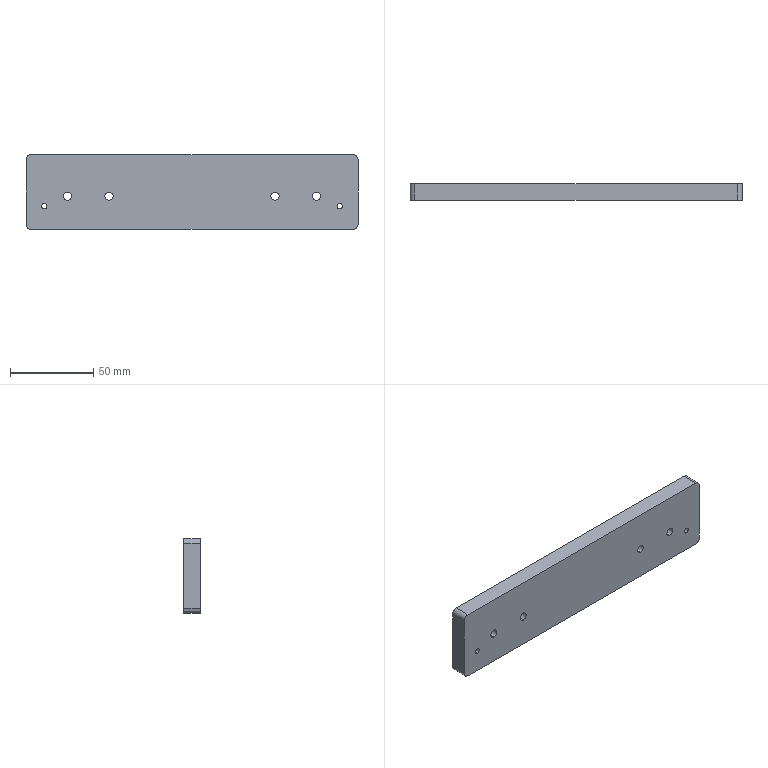Part | SolidWorks | features HoleWzd 2, MoveFace 2, Extrusion 1, Fillet 1 | 1 solid | 22 faces | box 200 x 10 x 45 mm | volume 88966 mm3 | cylinder 16 | plane 6 | commonest cylinder face diameters 5 x8 3.3 x4 6 x4
STEP:
#1=CARTESIAN_POINT('',(-75.,0.,-2.5));
#2=VERTEX_POINT('',#1);
#3=CARTESIAN_POINT('',(-75.,0.,2.5));
#4=VERTEX_POINT('',#3);
#5=CARTESIAN_POINT('',(-75.,0.,0.));
#6=DIRECTION('',(0.,1.,0.));
#7=DIRECTION('',(0.,0.,1.));
#8=AXIS2_PLACEMENT_3D('',#5,#6,#7);
#9=CIRCLE('',#8,2.5);
#10=EDGE_CURVE('',#2,#4,#9,.T.);
#11=ORIENTED_EDGE('',*,*,#10,.F.);
#12=CARTESIAN_POINT('',(-75.,10.,-2.5));
#13=VERTEX_POINT('',#12);
#14=CARTESIAN_POINT('',(-75.,10.,-2.5));
#15=DIRECTION('',(0.,1.,0.));
#16=VECTOR('',#15,1000.);
#17=LINE('',#14,#16);
#18=EDGE_CURVE('',#2,#13,#17,.T.);
#19=ORIENTED_EDGE('',*,*,#18,.T.);
#20=CARTESIAN_POINT('',(-75.,10.,2.5));
#21=VERTEX_POINT('',#20);
#22=CARTESIAN_POINT('',(-75.,10.,0.));
#23=DIRECTION('',(0.,1.,0.));
#24=DIRECTION('',(0.,0.,1.));
#25=AXIS2_PLACEMENT_3D('',#22,#23,#24);
#26=CIRCLE('',#25,2.5);
#27=EDGE_CURVE('',#13,#21,#26,.T.);
#28=ORIENTED_EDGE('',*,*,#27,.T.);
#29=CARTESIAN_POINT('',(-75.,10.,2.5));
#30=DIRECTION('',(0.,1.,0.));
#31=VECTOR('',#30,1000.);
#32=LINE('',#29,#31);
#33=EDGE_CURVE('',#4,#21,#32,.T.);
#34=ORIENTED_EDGE('',*,*,#33,.F.);
#35=EDGE_LOOP('',(#11,#19,#28,#34));
#36=FACE_OUTER_BOUND('',#35,.T.);
#37=CARTESIAN_POINT('',(-75.,10.,0.));
#38=DIRECTION('',(0.,1.,0.));
#39=DIRECTION('',(0.,0.,1.));
#40=AXIS2_PLACEMENT_3D('',#37,#38,#39);
#41=CYLINDRICAL_SURFACE('',#40,2.5);
#42=ADVANCED_FACE('',(#36),#41,.F.);
#43=CARTESIAN_POINT('',(75.,0.,-2.5));
#44=VERTEX_POINT('',#43);
#45=CARTESIAN_POINT('',(75.,0.,2.5));
#46=VERTEX_POINT('',#45);
#47=CARTESIAN_POINT('',(75.,0.,0.));
#48=DIRECTION('',(0.,1.,0.));
#49=DIRECTION('',(0.,0.,1.));
#50=AXIS2_PLACEMENT_3D('',#47,#48,#49);
#51=CIRCLE('',#50,2.5);
#52=EDGE_CURVE('',#44,#46,#51,.T.);
#53=ORIENTED_EDGE('',*,*,#52,.F.);
#54=CARTESIAN_POINT('',(75.,10.,-2.5));
#55=VERTEX_POINT('',#54);
#56=CARTESIAN_POINT('',(75.,10.,-2.5));
#57=DIRECTION('',(0.,1.,0.));
#58=VECTOR('',#57,1000.);
#59=LINE('',#56,#58);
#60=EDGE_CURVE('',#44,#55,#59,.T.);
#61=ORIENTED_EDGE('',*,*,#60,.T.);
#62=CARTESIAN_POINT('',(75.,10.,2.5));
#63=VERTEX_POINT('',#62);
#64=CARTESIAN_POINT('',(75.,10.,0.));
#65=DIRECTION('',(0.,1.,0.));
#66=DIRECTION('',(0.,0.,1.));
#67=AXIS2_PLACEMENT_3D('',#64,#65,#66);
#68=CIRCLE('',#67,2.5);
#69=EDGE_CURVE('',#55,#63,#68,.T.);
#70=ORIENTED_EDGE('',*,*,#69,.T.);
#71=CARTESIAN_POINT('',(75.,10.,2.5));
#72=DIRECTION('',(0.,1.,0.));
#73=VECTOR('',#72,1000.);
#74=LINE('',#71,#73);
#75=EDGE_CURVE('',#46,#63,#74,.T.);
#76=ORIENTED_EDGE('',*,*,#75,.F.);
#77=EDGE_LOOP('',(#53,#61,#70,#76));
#78=FACE_OUTER_BOUND('',#77,.T.);
#79=CARTESIAN_POINT('',(75.,10.,0.));
#80=DIRECTION('',(0.,1.,0.));
#81=DIRECTION('',(0.,0.,1.));
#82=AXIS2_PLACEMENT_3D('',#79,#80,#81);
#83=CYLINDRICAL_SURFACE('',#82,2.5);
#84=ADVANCED_FACE('',(#78),#83,.F.);
#85=CARTESIAN_POINT('',(-50.,0.,-2.5));
#86=VERTEX_POINT('',#85);
#87=CARTESIAN_POINT('',(-50.,0.,2.5));
#88=VERTEX_POINT('',#87);
#89=CARTESIAN_POINT('',(-50.,0.,0.));
#90=DIRECTION('',(0.,1.,0.));
#91=DIRECTION('',(0.,0.,1.));
#92=AXIS2_PLACEMENT_3D('',#89,#90,#91);
#93=CIRCLE('',#92,2.5);
#94=EDGE_CURVE('',#86,#88,#93,.T.);
#95=ORIENTED_EDGE('',*,*,#94,.F.);
#96=CARTESIAN_POINT('',(-50.,10.,-2.5));
#97=VERTEX_POINT('',#96);
#98=CARTESIAN_POINT('',(-50.,10.,-2.5));
#99=DIRECTION('',(0.,1.,0.));
#100=VECTOR('',#99,1000.);
#101=LINE('',#98,#100);
#102=EDGE_CURVE('',#86,#97,#101,.T.);
#103=ORIENTED_EDGE('',*,*,#102,.T.);
#104=CARTESIAN_POINT('',(-50.,10.,2.5));
#105=VERTEX_POINT('',#104);
#106=CARTESIAN_POINT('',(-50.,10.,0.));
#107=DIRECTION('',(0.,1.,0.));
#108=DIRECTION('',(0.,0.,1.));
#109=AXIS2_PLACEMENT_3D('',#106,#107,#108);
#110=CIRCLE('',#109,2.5);
#111=EDGE_CURVE('',#97,#105,#110,.T.);
#112=ORIENTED_EDGE('',*,*,#111,.T.);
#113=CARTESIAN_POINT('',(-50.,10.,2.5));
#114=DIRECTION('',(0.,1.,0.));
#115=VECTOR('',#114,1000.);
#116=LINE('',#113,#115);
#117=EDGE_CURVE('',#88,#105,#116,.T.);
#118=ORIENTED_EDGE('',*,*,#117,.F.);
#119=EDGE_LOOP('',(#95,#103,#112,#118));
#120=FACE_OUTER_BOUND('',#119,.T.);
#121=CARTESIAN_POINT('',(-50.,10.,0.));
#122=DIRECTION('',(0.,1.,0.));
#123=DIRECTION('',(0.,0.,1.));
#124=AXIS2_PLACEMENT_3D('',#121,#122,#123);
#125=CYLINDRICAL_SURFACE('',#124,2.5);
#126=ADVANCED_FACE('',(#120),#125,.F.);
#127=CARTESIAN_POINT('',(50.,0.,-2.5));
#128=VERTEX_POINT('',#127);
#129=CARTESIAN_POINT('',(50.,0.,2.5));
#130=VERTEX_POINT('',#129);
#131=CARTESIAN_POINT('',(50.,0.,0.));
#132=DIRECTION('',(0.,1.,0.));
#133=DIRECTION('',(0.,0.,1.));
#134=AXIS2_PLACEMENT_3D('',#131,#132,#133);
#135=CIRCLE('',#134,2.5);
#136=EDGE_CURVE('',#128,#130,#135,.T.);
#137=ORIENTED_EDGE('',*,*,#136,.F.);
#138=CARTESIAN_POINT('',(50.,10.,-2.5));
#139=VERTEX_POINT('',#138);
#140=CARTESIAN_POINT('',(50.,10.,-2.5));
#141=DIRECTION('',(0.,1.,0.));
#142=VECTOR('',#141,1000.);
#143=LINE('',#140,#142);
#144=EDGE_CURVE('',#128,#139,#143,.T.);
#145=ORIENTED_EDGE('',*,*,#144,.T.);
#146=CARTESIAN_POINT('',(50.,10.,2.5));
#147=VERTEX_POINT('',#146);
#148=CARTESIAN_POINT('',(50.,10.,0.));
#149=DIRECTION('',(0.,1.,0.));
#150=DIRECTION('',(0.,0.,1.));
#151=AXIS2_PLACEMENT_3D('',#148,#149,#150);
#152=CIRCLE('',#151,2.5);
#153=EDGE_CURVE('',#139,#147,#152,.T.);
#154=ORIENTED_EDGE('',*,*,#153,.T.);
#155=CARTESIAN_POINT('',(50.,10.,2.5));
#156=DIRECTION('',(0.,1.,0.));
#157=VECTOR('',#156,1000.);
#158=LINE('',#155,#157);
#159=EDGE_CURVE('',#130,#147,#158,.T.);
#160=ORIENTED_EDGE('',*,*,#159,.F.);
#161=EDGE_LOOP('',(#137,#145,#154,#160));
#162=FACE_OUTER_BOUND('',#161,.T.);
#163=CARTESIAN_POINT('',(50.,10.,0.));
#164=DIRECTION('',(0.,1.,0.));
#165=DIRECTION('',(0.,0.,1.));
#166=AXIS2_PLACEMENT_3D('',#163,#164,#165);
#167=CYLINDRICAL_SURFACE('',#166,2.5);
#168=ADVANCED_FACE('',(#162),#167,.F.);
#169=CARTESIAN_POINT('',(-89.,0.,-7.65));
#170=VERTEX_POINT('',#169);
#171=CARTESIAN_POINT('',(-89.,0.,-4.35));
#172=VERTEX_POINT('',#171);
#173=CARTESIAN_POINT('',(-89.,0.,-6.));
#174=DIRECTION('',(0.,1.,0.));
#175=DIRECTION('',(0.,0.,1.));
#176=AXIS2_PLACEMENT_3D('',#173,#174,#175);
#177=CIRCLE('',#176,1.65);
#178=EDGE_CURVE('',#170,#172,#177,.T.);
#179=ORIENTED_EDGE('',*,*,#178,.F.);
#180=CARTESIAN_POINT('',(-89.,10.,-7.65));
#181=VERTEX_POINT('',#180);
#182=CARTESIAN_POINT('',(-89.,10.,-7.65));
#183=DIRECTION('',(0.,1.,0.));
#184=VECTOR('',#183,1000.);
#185=LINE('',#182,#184);
#186=EDGE_CURVE('',#170,#181,#185,.T.);
#187=ORIENTED_EDGE('',*,*,#186,.T.);
#188=CARTESIAN_POINT('',(-89.,10.,-4.35));
#189=VERTEX_POINT('',#188);
#190=CARTESIAN_POINT('',(-89.,10.,-6.));
#191=DIRECTION('',(0.,1.,0.));
#192=DIRECTION('',(0.,0.,1.));
#193=AXIS2_PLACEMENT_3D('',#190,#191,#192);
#194=CIRCLE('',#193,1.65);
#195=EDGE_CURVE('',#181,#189,#194,.T.);
#196=ORIENTED_EDGE('',*,*,#195,.T.);
#197=CARTESIAN_POINT('',(-89.,10.,-4.35));
#198=DIRECTION('',(0.,1.,0.));
#199=VECTOR('',#198,1000.);
#200=LINE('',#197,#199);
#201=EDGE_CURVE('',#172,#189,#200,.T.);
#202=ORIENTED_EDGE('',*,*,#201,.F.);
#203=EDGE_LOOP('',(#179,#187,#196,#202));
#204=FACE_OUTER_BOUND('',#203,.T.);
#205=CARTESIAN_POINT('',(-89.,10.,-6.));
#206=DIRECTION('',(0.,1.,0.));
#207=DIRECTION('',(0.,0.,1.));
#208=AXIS2_PLACEMENT_3D('',#205,#206,#207);
#209=CYLINDRICAL_SURFACE('',#208,1.65);
#210=ADVANCED_FACE('',(#204),#209,.F.);
#211=CARTESIAN_POINT('',(89.,0.,-7.65));
#212=VERTEX_POINT('',#211);
#213=CARTESIAN_POINT('',(89.,0.,-4.35));
#214=VERTEX_POINT('',#213);
#215=CARTESIAN_POINT('',(89.,0.,-6.));
#216=DIRECTION('',(0.,1.,0.));
#217=DIRECTION('',(0.,0.,1.));
#218=AXIS2_PLACEMENT_3D('',#215,#216,#217);
#219=CIRCLE('',#218,1.65);
#220=EDGE_CURVE('',#212,#214,#219,.T.);
#221=ORIENTED_EDGE('',*,*,#220,.F.);
#222=CARTESIAN_POINT('',(89.,10.,-7.65));
#223=VERTEX_POINT('',#222);
#224=CARTESIAN_POINT('',(89.,10.,-7.65));
#225=DIRECTION('',(0.,1.,0.));
#226=VECTOR('',#225,1000.);
#227=LINE('',#224,#226);
#228=EDGE_CURVE('',#212,#223,#227,.T.);
#229=ORIENTED_EDGE('',*,*,#228,.T.);
#230=CARTESIAN_POINT('',(89.,10.,-4.35));
#231=VERTEX_POINT('',#230);
#232=CARTESIAN_POINT('',(89.,10.,-6.));
#233=DIRECTION('',(0.,1.,0.));
#234=DIRECTION('',(0.,0.,1.));
#235=AXIS2_PLACEMENT_3D('',#232,#233,#234);
#236=CIRCLE('',#235,1.65);
#237=EDGE_CURVE('',#223,#231,#236,.T.);
#238=ORIENTED_EDGE('',*,*,#237,.T.);
#239=CARTESIAN_POINT('',(89.,10.,-4.35));
#240=DIRECTION('',(0.,1.,0.));
#241=VECTOR('',#240,1000.);
#242=LINE('',#239,#241);
#243=EDGE_CURVE('',#214,#231,#242,.T.);
#244=ORIENTED_EDGE('',*,*,#243,.F.);
#245=EDGE_LOOP('',(#221,#229,#238,#244));
#246=FACE_OUTER_BOUND('',#245,.T.);
#247=CARTESIAN_POINT('',(89.,10.,-6.));
#248=DIRECTION('',(0.,1.,0.));
#249=DIRECTION('',(0.,0.,1.));
#250=AXIS2_PLACEMENT_3D('',#247,#248,#249);
#251=CYLINDRICAL_SURFACE('',#250,1.65);
#252=ADVANCED_FACE('',(#246),#251,.F.);
#253=CARTESIAN_POINT('',(-75.,10.,0.));
#254=DIRECTION('',(0.,1.,0.));
#255=DIRECTION('',(0.,0.,1.));
#256=AXIS2_PLACEMENT_3D('',#253,#254,#255);
#257=CIRCLE('',#256,2.5);
#258=EDGE_CURVE('',#21,#13,#257,.T.);
#259=ORIENTED_EDGE('',*,*,#258,.F.);
#260=ORIENTED_EDGE('',*,*,#27,.F.);
#261=EDGE_LOOP('',(#259,#260));
#262=FACE_BOUND('',#261,.T.);
#263=CARTESIAN_POINT('',(75.,10.,0.));
#264=DIRECTION('',(0.,1.,0.));
#265=DIRECTION('',(0.,0.,1.));
#266=AXIS2_PLACEMENT_3D('',#263,#264,#265);
#267=CIRCLE('',#266,2.5);
#268=EDGE_CURVE('',#63,#55,#267,.T.);
#269=ORIENTED_EDGE('',*,*,#268,.F.);
#270=ORIENTED_EDGE('',*,*,#69,.F.);
#271=EDGE_LOOP('',(#269,#270));
#272=FACE_BOUND('',#271,.T.);
#273=CARTESIAN_POINT('',(-50.,10.,0.));
#274=DIRECTION('',(0.,1.,0.));
#275=DIRECTION('',(0.,0.,1.));
#276=AXIS2_PLACEMENT_3D('',#273,#274,#275);
#277=CIRCLE('',#276,2.5);
#278=EDGE_CURVE('',#105,#97,#277,.T.);
#279=ORIENTED_EDGE('',*,*,#278,.F.);
#280=ORIENTED_EDGE('',*,*,#111,.F.);
#281=EDGE_LOOP('',(#279,#280));
#282=FACE_BOUND('',#281,.T.);
#283=CARTESIAN_POINT('',(50.,10.,0.));
#284=DIRECTION('',(0.,1.,0.));
#285=DIRECTION('',(0.,0.,1.));
#286=AXIS2_PLACEMENT_3D('',#283,#284,#285);
#287=CIRCLE('',#286,2.5);
#288=EDGE_CURVE('',#147,#139,#287,.T.);
#289=ORIENTED_EDGE('',*,*,#288,.F.);
#290=ORIENTED_EDGE('',*,*,#153,.F.);
#291=EDGE_LOOP('',(#289,#290));
#292=FACE_BOUND('',#291,.T.);
#293=CARTESIAN_POINT('',(89.,10.,-6.));
#294=DIRECTION('',(0.,1.,0.));
#295=DIRECTION('',(0.,0.,1.));
#296=AXIS2_PLACEMENT_3D('',#293,#294,#295);
#297=CIRCLE('',#296,1.65);
#298=EDGE_CURVE('',#231,#223,#297,.T.);
#299=ORIENTED_EDGE('',*,*,#298,.F.);
#300=ORIENTED_EDGE('',*,*,#237,.F.);
#301=EDGE_LOOP('',(#299,#300));
#302=FACE_BOUND('',#301,.T.);
#303=CARTESIAN_POINT('',(100.,10.,22.));
#304=VERTEX_POINT('',#303);
#305=CARTESIAN_POINT('',(100.,10.,-17.));
#306=VERTEX_POINT('',#305);
#307=CARTESIAN_POINT('',(100.,10.,10.));
#308=DIRECTION('',(0.,0.,-1.));
#309=VECTOR('',#308,1000.);
#310=LINE('',#307,#309);
#311=EDGE_CURVE('',#304,#306,#310,.T.);
#312=ORIENTED_EDGE('',*,*,#311,.T.);
#313=CARTESIAN_POINT('',(97.,10.,-20.));
#314=VERTEX_POINT('',#313);
#315=CARTESIAN_POINT('',(97.,10.,-17.));
#316=DIRECTION('',(0.,1.,0.));
#317=DIRECTION('',(0.,0.,-1.));
#318=AXIS2_PLACEMENT_3D('',#315,#316,#317);
#319=CIRCLE('',#318,3.);
#320=EDGE_CURVE('',#306,#314,#319,.T.);
#321=ORIENTED_EDGE('',*,*,#320,.T.);
#322=CARTESIAN_POINT('',(-97.,10.,-20.));
#323=VERTEX_POINT('',#322);
#324=CARTESIAN_POINT('',(-100.,10.,-20.));
#325=DIRECTION('',(-1.,0.,0.));
#326=VECTOR('',#325,1000.);
#327=LINE('',#324,#326);
#328=EDGE_CURVE('',#314,#323,#327,.T.);
#329=ORIENTED_EDGE('',*,*,#328,.T.);
#330=CARTESIAN_POINT('',(-100.,10.,-17.));
#331=VERTEX_POINT('',#330);
#332=CARTESIAN_POINT('',(-97.,10.,-17.));
#333=DIRECTION('',(0.,1.,0.));
#334=DIRECTION('',(0.,0.,-1.));
#335=AXIS2_PLACEMENT_3D('',#332,#333,#334);
#336=CIRCLE('',#335,3.);
#337=EDGE_CURVE('',#323,#331,#336,.T.);
#338=ORIENTED_EDGE('',*,*,#337,.T.);
#339=CARTESIAN_POINT('',(-100.,10.,22.));
#340=VERTEX_POINT('',#339);
#341=CARTESIAN_POINT('',(-100.,10.,10.));
#342=DIRECTION('',(0.,0.,1.));
#343=VECTOR('',#342,1000.);
#344=LINE('',#341,#343);
#345=EDGE_CURVE('',#331,#340,#344,.T.);
#346=ORIENTED_EDGE('',*,*,#345,.T.);
#347=CARTESIAN_POINT('',(-97.,10.,25.));
#348=VERTEX_POINT('',#347);
#349=CARTESIAN_POINT('',(-97.,10.,22.));
#350=DIRECTION('',(0.,1.,0.));
#351=DIRECTION('',(0.,0.,-1.));
#352=AXIS2_PLACEMENT_3D('',#349,#350,#351);
#353=CIRCLE('',#352,3.);
#354=EDGE_CURVE('',#340,#348,#353,.T.);
#355=ORIENTED_EDGE('',*,*,#354,.T.);
#356=CARTESIAN_POINT('',(97.,10.,25.));
#357=VERTEX_POINT('',#356);
#358=CARTESIAN_POINT('',(-100.,10.,25.));
#359=DIRECTION('',(1.,0.,0.));
#360=VECTOR('',#359,1000.);
#361=LINE('',#358,#360);
#362=EDGE_CURVE('',#348,#357,#361,.T.);
#363=ORIENTED_EDGE('',*,*,#362,.T.);
#364=CARTESIAN_POINT('',(97.,10.,22.));
#365=DIRECTION('',(0.,1.,0.));
#366=DIRECTION('',(0.,0.,-1.));
#367=AXIS2_PLACEMENT_3D('',#364,#365,#366);
#368=CIRCLE('',#367,3.);
#369=EDGE_CURVE('',#357,#304,#368,.T.);
#370=ORIENTED_EDGE('',*,*,#369,.T.);
#371=EDGE_LOOP('',(#312,#321,#329,#338,#346,#355,#363,#370));
#372=FACE_OUTER_BOUND('',#371,.T.);
#373=CARTESIAN_POINT('',(-89.,10.,-6.));
#374=DIRECTION('',(0.,1.,0.));
#375=DIRECTION('',(0.,0.,1.));
#376=AXIS2_PLACEMENT_3D('',#373,#374,#375);
#377=CIRCLE('',#376,1.65);
#378=EDGE_CURVE('',#189,#181,#377,.T.);
#379=ORIENTED_EDGE('',*,*,#378,.F.);
#380=ORIENTED_EDGE('',*,*,#195,.F.);
#381=EDGE_LOOP('',(#379,#380));
#382=FACE_BOUND('',#381,.T.);
#383=CARTESIAN_POINT('',(0.,10.,0.));
#384=DIRECTION('',(0.,-1.,0.));
#385=DIRECTION('',(0.,0.,-1.));
#386=AXIS2_PLACEMENT_3D('',#383,#384,#385);
#387=PLANE('',#386);
#388=ADVANCED_FACE('',(#262,#272,#282,#292,#302,#372,#382),#387,.F.);
#389=CARTESIAN_POINT('',(100.,0.,22.));
#390=VERTEX_POINT('',#389);
#391=CARTESIAN_POINT('',(100.,0.,-17.));
#392=VERTEX_POINT('',#391);
#393=CARTESIAN_POINT('',(100.,0.,10.));
#394=DIRECTION('',(0.,0.,-1.));
#395=VECTOR('',#394,1000.);
#396=LINE('',#393,#395);
#397=EDGE_CURVE('',#390,#392,#396,.T.);
#398=ORIENTED_EDGE('',*,*,#397,.T.);
#399=CARTESIAN_POINT('',(100.,10.,-17.));
#400=DIRECTION('',(0.,1.,0.));
#401=VECTOR('',#400,1000.);
#402=LINE('',#399,#401);
#403=EDGE_CURVE('',#392,#306,#402,.T.);
#404=ORIENTED_EDGE('',*,*,#403,.T.);
#405=ORIENTED_EDGE('',*,*,#311,.F.);
#406=CARTESIAN_POINT('',(100.,10.,22.));
#407=DIRECTION('',(0.,-1.,0.));
#408=VECTOR('',#407,1000.);
#409=LINE('',#406,#408);
#410=EDGE_CURVE('',#304,#390,#409,.T.);
#411=ORIENTED_EDGE('',*,*,#410,.T.);
#412=EDGE_LOOP('',(#398,#404,#405,#411));
#413=FACE_OUTER_BOUND('',#412,.T.);
#414=CARTESIAN_POINT('',(100.,10.,10.));
#415=DIRECTION('',(-1.,0.,0.));
#416=DIRECTION('',(0.,0.,1.));
#417=AXIS2_PLACEMENT_3D('',#414,#415,#416);
#418=PLANE('',#417);
#419=ADVANCED_FACE('',(#413),#418,.F.);
#420=ORIENTED_EDGE('',*,*,#328,.F.);
#421=CARTESIAN_POINT('',(97.,0.,-20.));
#422=VERTEX_POINT('',#421);
#423=CARTESIAN_POINT('',(97.,10.,-20.));
#424=DIRECTION('',(0.,-1.,0.));
#425=VECTOR('',#424,1000.);
#426=LINE('',#423,#425);
#427=EDGE_CURVE('',#314,#422,#426,.T.);
#428=ORIENTED_EDGE('',*,*,#427,.T.);
#429=CARTESIAN_POINT('',(-97.,0.,-20.));
#430=VERTEX_POINT('',#429);
#431=CARTESIAN_POINT('',(-100.,0.,-20.));
#432=DIRECTION('',(-1.,0.,0.));
#433=VECTOR('',#432,1000.);
#434=LINE('',#431,#433);
#435=EDGE_CURVE('',#422,#430,#434,.T.);
#436=ORIENTED_EDGE('',*,*,#435,.T.);
#437=CARTESIAN_POINT('',(-97.,10.,-20.));
#438=DIRECTION('',(0.,1.,0.));
#439=VECTOR('',#438,1000.);
#440=LINE('',#437,#439);
#441=EDGE_CURVE('',#430,#323,#440,.T.);
#442=ORIENTED_EDGE('',*,*,#441,.T.);
#443=EDGE_LOOP('',(#420,#428,#436,#442));
#444=FACE_OUTER_BOUND('',#443,.T.);
#445=CARTESIAN_POINT('',(-100.,10.,-20.));
#446=DIRECTION('',(0.,0.,1.));
#447=DIRECTION('',(1.,0.,0.));
#448=AXIS2_PLACEMENT_3D('',#445,#446,#447);
#449=PLANE('',#448);
#450=ADVANCED_FACE('',(#444),#449,.F.);
#451=ORIENTED_EDGE('',*,*,#345,.F.);
#452=CARTESIAN_POINT('',(-100.,0.,-17.));
#453=VERTEX_POINT('',#452);
#454=CARTESIAN_POINT('',(-100.,10.,-17.));
#455=DIRECTION('',(0.,-1.,0.));
#456=VECTOR('',#455,1000.);
#457=LINE('',#454,#456);
#458=EDGE_CURVE('',#331,#453,#457,.T.);
#459=ORIENTED_EDGE('',*,*,#458,.T.);
#460=CARTESIAN_POINT('',(-100.,0.,22.));
#461=VERTEX_POINT('',#460);
#462=CARTESIAN_POINT('',(-100.,0.,10.));
#463=DIRECTION('',(0.,0.,1.));
#464=VECTOR('',#463,1000.);
#465=LINE('',#462,#464);
#466=EDGE_CURVE('',#453,#461,#465,.T.);
#467=ORIENTED_EDGE('',*,*,#466,.T.);
#468=CARTESIAN_POINT('',(-100.,10.,22.));
#469=DIRECTION('',(0.,1.,0.));
#470=VECTOR('',#469,1000.);
#471=LINE('',#468,#470);
#472=EDGE_CURVE('',#461,#340,#471,.T.);
#473=ORIENTED_EDGE('',*,*,#472,.T.);
#474=EDGE_LOOP('',(#451,#459,#467,#473));
#475=FACE_OUTER_BOUND('',#474,.T.);
#476=CARTESIAN_POINT('',(-100.,10.,10.));
#477=DIRECTION('',(1.,0.,0.));
#478=DIRECTION('',(0.,0.,-1.));
#479=AXIS2_PLACEMENT_3D('',#476,#477,#478);
#480=PLANE('',#479);
#481=ADVANCED_FACE('',(#475),#480,.F.);
#482=CARTESIAN_POINT('',(-97.,0.,25.));
#483=VERTEX_POINT('',#482);
#484=CARTESIAN_POINT('',(97.,0.,25.));
#485=VERTEX_POINT('',#484);
#486=CARTESIAN_POINT('',(-100.,0.,25.));
#487=DIRECTION('',(1.,0.,0.));
#488=VECTOR('',#487,1000.);
#489=LINE('',#486,#488);
#490=EDGE_CURVE('',#483,#485,#489,.T.);
#491=ORIENTED_EDGE('',*,*,#490,.T.);
#492=CARTESIAN_POINT('',(97.,10.,25.));
#493=DIRECTION('',(0.,1.,0.));
#494=VECTOR('',#493,1000.);
#495=LINE('',#492,#494);
#496=EDGE_CURVE('',#485,#357,#495,.T.);
#497=ORIENTED_EDGE('',*,*,#496,.T.);
#498=ORIENTED_EDGE('',*,*,#362,.F.);
#499=CARTESIAN_POINT('',(-97.,10.,25.));
#500=DIRECTION('',(0.,-1.,0.));
#501=VECTOR('',#500,1000.);
#502=LINE('',#499,#501);
#503=EDGE_CURVE('',#348,#483,#502,.T.);
#504=ORIENTED_EDGE('',*,*,#503,.T.);
#505=EDGE_LOOP('',(#491,#497,#498,#504));
#506=FACE_OUTER_BOUND('',#505,.T.);
#507=CARTESIAN_POINT('',(-100.,10.,25.));
#508=DIRECTION('',(0.,0.,-1.));
#509=DIRECTION('',(-1.,0.,0.));
#510=AXIS2_PLACEMENT_3D('',#507,#508,#509);
#511=PLANE('',#510);
#512=ADVANCED_FACE('',(#506),#511,.F.);
#513=CARTESIAN_POINT('',(-75.,0.,0.));
#514=DIRECTION('',(0.,1.,0.));
#515=DIRECTION('',(0.,0.,1.));
#516=AXIS2_PLACEMENT_3D('',#513,#514,#515);
#517=CIRCLE('',#516,2.5);
#518=EDGE_CURVE('',#4,#2,#517,.T.);
#519=ORIENTED_EDGE('',*,*,#518,.T.);
#520=ORIENTED_EDGE('',*,*,#10,.T.);
#521=EDGE_LOOP('',(#519,#520));
#522=FACE_BOUND('',#521,.T.);
#523=CARTESIAN_POINT('',(75.,0.,0.));
#524=DIRECTION('',(0.,1.,0.));
#525=DIRECTION('',(0.,0.,1.));
#526=AXIS2_PLACEMENT_3D('',#523,#524,#525);
#527=CIRCLE('',#526,2.5);
#528=EDGE_CURVE('',#46,#44,#527,.T.);
#529=ORIENTED_EDGE('',*,*,#528,.T.);
#530=ORIENTED_EDGE('',*,*,#52,.T.);
#531=EDGE_LOOP('',(#529,#530));
#532=FACE_BOUND('',#531,.T.);
#533=CARTESIAN_POINT('',(-50.,0.,0.));
#534=DIRECTION('',(0.,1.,0.));
#535=DIRECTION('',(0.,0.,1.));
#536=AXIS2_PLACEMENT_3D('',#533,#534,#535);
#537=CIRCLE('',#536,2.5);
#538=EDGE_CURVE('',#88,#86,#537,.T.);
#539=ORIENTED_EDGE('',*,*,#538,.T.);
#540=ORIENTED_EDGE('',*,*,#94,.T.);
#541=EDGE_LOOP('',(#539,#540));
#542=FACE_BOUND('',#541,.T.);
#543=CARTESIAN_POINT('',(50.,0.,0.));
#544=DIRECTION('',(0.,1.,0.));
#545=DIRECTION('',(0.,0.,1.));
#546=AXIS2_PLACEMENT_3D('',#543,#544,#545);
#547=CIRCLE('',#546,2.5);
#548=EDGE_CURVE('',#130,#128,#547,.T.);
#549=ORIENTED_EDGE('',*,*,#548,.T.);
#550=ORIENTED_EDGE('',*,*,#136,.T.);
#551=EDGE_LOOP('',(#549,#550));
#552=FACE_BOUND('',#551,.T.);
#553=CARTESIAN_POINT('',(-89.,0.,-6.));
#554=DIRECTION('',(0.,1.,0.));
#555=DIRECTION('',(0.,0.,1.));
#556=AXIS2_PLACEMENT_3D('',#553,#554,#555);
#557=CIRCLE('',#556,1.65);
#558=EDGE_CURVE('',#172,#170,#557,.T.);
#559=ORIENTED_EDGE('',*,*,#558,.T.);
#560=ORIENTED_EDGE('',*,*,#178,.T.);
#561=EDGE_LOOP('',(#559,#560));
#562=FACE_BOUND('',#561,.T.);
#563=CARTESIAN_POINT('',(89.,0.,-6.));
#564=DIRECTION('',(0.,1.,0.));
#565=DIRECTION('',(0.,0.,1.));
#566=AXIS2_PLACEMENT_3D('',#563,#564,#565);
#567=CIRCLE('',#566,1.65);
#568=EDGE_CURVE('',#214,#212,#567,.T.);
#569=ORIENTED_EDGE('',*,*,#568,.T.);
#570=ORIENTED_EDGE('',*,*,#220,.T.);
#571=EDGE_LOOP('',(#569,#570));
#572=FACE_BOUND('',#571,.T.);
#573=ORIENTED_EDGE('',*,*,#435,.F.);
#574=CARTESIAN_POINT('',(97.,0.,-17.));
#575=DIRECTION('',(0.,-1.,0.));
#576=DIRECTION('',(0.,0.,-1.));
#577=AXIS2_PLACEMENT_3D('',#574,#575,#576);
#578=CIRCLE('',#577,3.);
#579=EDGE_CURVE('',#422,#392,#578,.T.);
#580=ORIENTED_EDGE('',*,*,#579,.T.);
#581=ORIENTED_EDGE('',*,*,#397,.F.);
#582=CARTESIAN_POINT('',(97.,0.,22.));
#583=DIRECTION('',(0.,-1.,0.));
#584=DIRECTION('',(0.,0.,-1.));
#585=AXIS2_PLACEMENT_3D('',#582,#583,#584);
#586=CIRCLE('',#585,3.);
#587=EDGE_CURVE('',#390,#485,#586,.T.);
#588=ORIENTED_EDGE('',*,*,#587,.T.);
#589=ORIENTED_EDGE('',*,*,#490,.F.);
#590=CARTESIAN_POINT('',(-97.,0.,22.));
#591=DIRECTION('',(0.,-1.,0.));
#592=DIRECTION('',(0.,0.,-1.));
#593=AXIS2_PLACEMENT_3D('',#590,#591,#592);
#594=CIRCLE('',#593,3.);
#595=EDGE_CURVE('',#483,#461,#594,.T.);
#596=ORIENTED_EDGE('',*,*,#595,.T.);
#597=ORIENTED_EDGE('',*,*,#466,.F.);
#598=CARTESIAN_POINT('',(-97.,0.,-17.));
#599=DIRECTION('',(0.,-1.,0.));
#600=DIRECTION('',(0.,0.,-1.));
#601=AXIS2_PLACEMENT_3D('',#598,#599,#600);
#602=CIRCLE('',#601,3.);
#603=EDGE_CURVE('',#453,#430,#602,.T.);
#604=ORIENTED_EDGE('',*,*,#603,.T.);
#605=EDGE_LOOP('',(#573,#580,#581,#588,#589,#596,#597,#604));
#606=FACE_OUTER_BOUND('',#605,.T.);
#607=CARTESIAN_POINT('',(0.,0.,0.));
#608=DIRECTION('',(0.,-1.,0.));
#609=DIRECTION('',(0.,0.,-1.));
#610=AXIS2_PLACEMENT_3D('',#607,#608,#609);
#611=PLANE('',#610);
#612=ADVANCED_FACE('',(#522,#532,#542,#552,#562,#572,#606),#611,.T.);
#613=ORIENTED_EDGE('',*,*,#320,.F.);
#614=ORIENTED_EDGE('',*,*,#403,.F.);
#615=ORIENTED_EDGE('',*,*,#579,.F.);
#616=ORIENTED_EDGE('',*,*,#427,.F.);
#617=EDGE_LOOP('',(#613,#614,#615,#616));
#618=FACE_OUTER_BOUND('',#617,.T.);
#619=CARTESIAN_POINT('',(97.,10.,-17.));
#620=DIRECTION('',(0.,-1.,0.));
#621=DIRECTION('',(0.,0.,-1.));
#622=AXIS2_PLACEMENT_3D('',#619,#620,#621);
#623=CYLINDRICAL_SURFACE('',#622,3.);
#624=ADVANCED_FACE('',(#618),#623,.T.);
#625=ORIENTED_EDGE('',*,*,#369,.F.);
#626=ORIENTED_EDGE('',*,*,#496,.F.);
#627=ORIENTED_EDGE('',*,*,#587,.F.);
#628=ORIENTED_EDGE('',*,*,#410,.F.);
#629=EDGE_LOOP('',(#625,#626,#627,#628));
#630=FACE_OUTER_BOUND('',#629,.T.);
#631=CARTESIAN_POINT('',(97.,10.,22.));
#632=DIRECTION('',(0.,-1.,0.));
#633=DIRECTION('',(0.,0.,-1.));
#634=AXIS2_PLACEMENT_3D('',#631,#632,#633);
#635=CYLINDRICAL_SURFACE('',#634,3.);
#636=ADVANCED_FACE('',(#630),#635,.T.);
#637=ORIENTED_EDGE('',*,*,#337,.F.);
#638=ORIENTED_EDGE('',*,*,#441,.F.);
#639=ORIENTED_EDGE('',*,*,#603,.F.);
#640=ORIENTED_EDGE('',*,*,#458,.F.);
#641=EDGE_LOOP('',(#637,#638,#639,#640));
#642=FACE_OUTER_BOUND('',#641,.T.);
#643=CARTESIAN_POINT('',(-97.,10.,-17.));
#644=DIRECTION('',(0.,-1.,0.));
#645=DIRECTION('',(0.,0.,-1.));
#646=AXIS2_PLACEMENT_3D('',#643,#644,#645);
#647=CYLINDRICAL_SURFACE('',#646,3.);
#648=ADVANCED_FACE('',(#642),#647,.T.);
#649=ORIENTED_EDGE('',*,*,#354,.F.);
#650=ORIENTED_EDGE('',*,*,#472,.F.);
#651=ORIENTED_EDGE('',*,*,#595,.F.);
#652=ORIENTED_EDGE('',*,*,#503,.F.);
#653=EDGE_LOOP('',(#649,#650,#651,#652));
#654=FACE_OUTER_BOUND('',#653,.T.);
#655=CARTESIAN_POINT('',(-97.,10.,22.));
#656=DIRECTION('',(0.,-1.,0.));
#657=DIRECTION('',(0.,0.,-1.));
#658=AXIS2_PLACEMENT_3D('',#655,#656,#657);
#659=CYLINDRICAL_SURFACE('',#658,3.);
#660=ADVANCED_FACE('',(#654),#659,.T.);
#661=ORIENTED_EDGE('',*,*,#228,.F.);
#662=ORIENTED_EDGE('',*,*,#568,.F.);
#663=ORIENTED_EDGE('',*,*,#243,.T.);
#664=ORIENTED_EDGE('',*,*,#298,.T.);
#665=EDGE_LOOP('',(#661,#662,#663,#664));
#666=FACE_OUTER_BOUND('',#665,.T.);
#667=CARTESIAN_POINT('',(89.,10.,-6.));
#668=DIRECTION('',(0.,1.,0.));
#669=DIRECTION('',(0.,0.,1.));
#670=AXIS2_PLACEMENT_3D('',#667,#668,#669);
#671=CYLINDRICAL_SURFACE('',#670,1.65);
#672=ADVANCED_FACE('',(#666),#671,.F.);
#673=ORIENTED_EDGE('',*,*,#186,.F.);
#674=ORIENTED_EDGE('',*,*,#558,.F.);
#675=ORIENTED_EDGE('',*,*,#201,.T.);
#676=ORIENTED_EDGE('',*,*,#378,.T.);
#677=EDGE_LOOP('',(#673,#674,#675,#676));
#678=FACE_OUTER_BOUND('',#677,.T.);
#679=CARTESIAN_POINT('',(-89.,10.,-6.));
#680=DIRECTION('',(0.,1.,0.));
#681=DIRECTION('',(0.,0.,1.));
#682=AXIS2_PLACEMENT_3D('',#679,#680,#681);
#683=CYLINDRICAL_SURFACE('',#682,1.65);
#684=ADVANCED_FACE('',(#678),#683,.F.);
#685=ORIENTED_EDGE('',*,*,#144,.F.);
#686=ORIENTED_EDGE('',*,*,#548,.F.);
#687=ORIENTED_EDGE('',*,*,#159,.T.);
#688=ORIENTED_EDGE('',*,*,#288,.T.);
#689=EDGE_LOOP('',(#685,#686,#687,#688));
#690=FACE_OUTER_BOUND('',#689,.T.);
#691=CARTESIAN_POINT('',(50.,10.,0.));
#692=DIRECTION('',(0.,1.,0.));
#693=DIRECTION('',(0.,0.,1.));
#694=AXIS2_PLACEMENT_3D('',#691,#692,#693);
#695=CYLINDRICAL_SURFACE('',#694,2.5);
#696=ADVANCED_FACE('',(#690),#695,.F.);
#697=ORIENTED_EDGE('',*,*,#102,.F.);
#698=ORIENTED_EDGE('',*,*,#538,.F.);
#699=ORIENTED_EDGE('',*,*,#117,.T.);
#700=ORIENTED_EDGE('',*,*,#278,.T.);
#701=EDGE_LOOP('',(#697,#698,#699,#700));
#702=FACE_OUTER_BOUND('',#701,.T.);
#703=CARTESIAN_POINT('',(-50.,10.,0.));
#704=DIRECTION('',(0.,1.,0.));
#705=DIRECTION('',(0.,0.,1.));
#706=AXIS2_PLACEMENT_3D('',#703,#704,#705);
#707=CYLINDRICAL_SURFACE('',#706,2.5);
#708=ADVANCED_FACE('',(#702),#707,.F.);
#709=ORIENTED_EDGE('',*,*,#60,.F.);
#710=ORIENTED_EDGE('',*,*,#528,.F.);
#711=ORIENTED_EDGE('',*,*,#75,.T.);
#712=ORIENTED_EDGE('',*,*,#268,.T.);
#713=EDGE_LOOP('',(#709,#710,#711,#712));
#714=FACE_OUTER_BOUND('',#713,.T.);
#715=CARTESIAN_POINT('',(75.,10.,0.));
#716=DIRECTION('',(0.,1.,0.));
#717=DIRECTION('',(0.,0.,1.));
#718=AXIS2_PLACEMENT_3D('',#715,#716,#717);
#719=CYLINDRICAL_SURFACE('',#718,2.5);
#720=ADVANCED_FACE('',(#714),#719,.F.);
#721=ORIENTED_EDGE('',*,*,#18,.F.);
#722=ORIENTED_EDGE('',*,*,#518,.F.);
#723=ORIENTED_EDGE('',*,*,#33,.T.);
#724=ORIENTED_EDGE('',*,*,#258,.T.);
#725=EDGE_LOOP('',(#721,#722,#723,#724));
#726=FACE_OUTER_BOUND('',#725,.T.);
#727=CARTESIAN_POINT('',(-75.,10.,0.));
#728=DIRECTION('',(0.,1.,0.));
#729=DIRECTION('',(0.,0.,1.));
#730=AXIS2_PLACEMENT_3D('',#727,#728,#729);
#731=CYLINDRICAL_SURFACE('',#730,2.5);
#732=ADVANCED_FACE('',(#726),#731,.F.);
#733=CLOSED_SHELL('',(#42,#84,#126,#168,#210,#252,#388,#419,#450,#481,#512,#612,#624,#636,#648,#660,#672,#684,#696,#708,#720,#732));
#734=MANIFOLD_SOLID_BREP('',#733);
#735=CARTESIAN_POINT('',(0.,0.,0.));
#736=DIRECTION('',(0.,0.,1.));
#737=DIRECTION('',(1.,0.,0.));
#738=AXIS2_PLACEMENT_3D('',#735,#736,#737);
#739=(LENGTH_UNIT()NAMED_UNIT(*)SI_UNIT(.MILLI.,.METRE.));
#740=UNCERTAINTY_MEASURE_WITH_UNIT(LENGTH_MEASURE(0.00001),#739,'','');
#741=(NAMED_UNIT(*)PLANE_ANGLE_UNIT()SI_UNIT($,.RADIAN.));
#742=(NAMED_UNIT(*)SI_UNIT($,.STERADIAN.)SOLID_ANGLE_UNIT());
#743=(GEOMETRIC_REPRESENTATION_CONTEXT(3)GLOBAL_UNCERTAINTY_ASSIGNED_CONTEXT((#740))GLOBAL_UNIT_ASSIGNED_CONTEXT((#739,#741,#742))REPRESENTATION_CONTEXT('',''));
#744=ADVANCED_BREP_SHAPE_REPRESENTATION('',(#734,#738),#743);